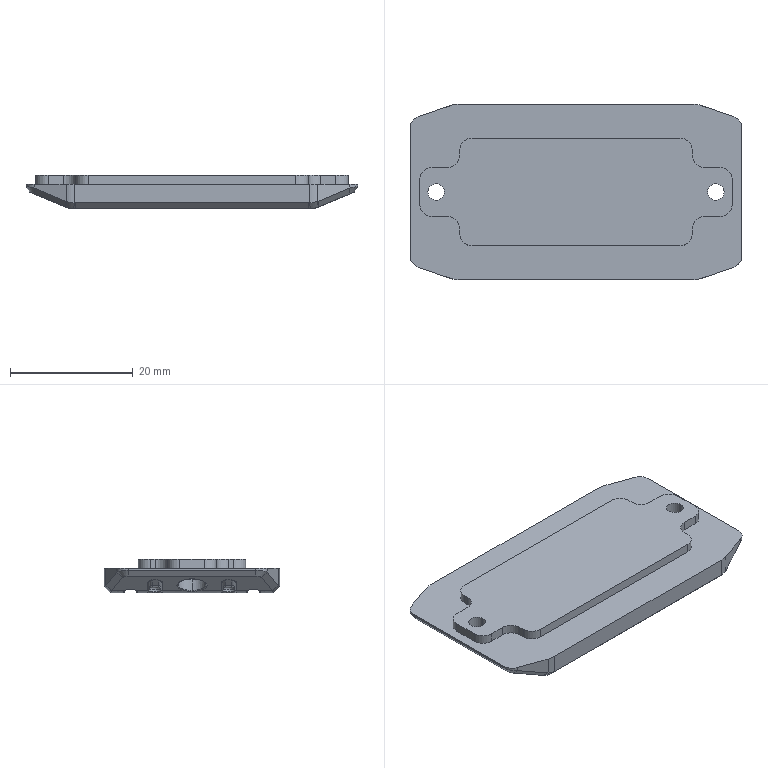Part | SolidWorks | features BaseBody 1 | 1 solid | 347 faces | box 54 x 28.5 x 5.5 mm | volume 5973 mm3 | cylinder 140 | plane 79 | torus 68 | spline 56 | cone 4 | commonest cylinder face diameters 2 x30 0.4 x28 1 x28 4 x16 8 x14 2.5 x8